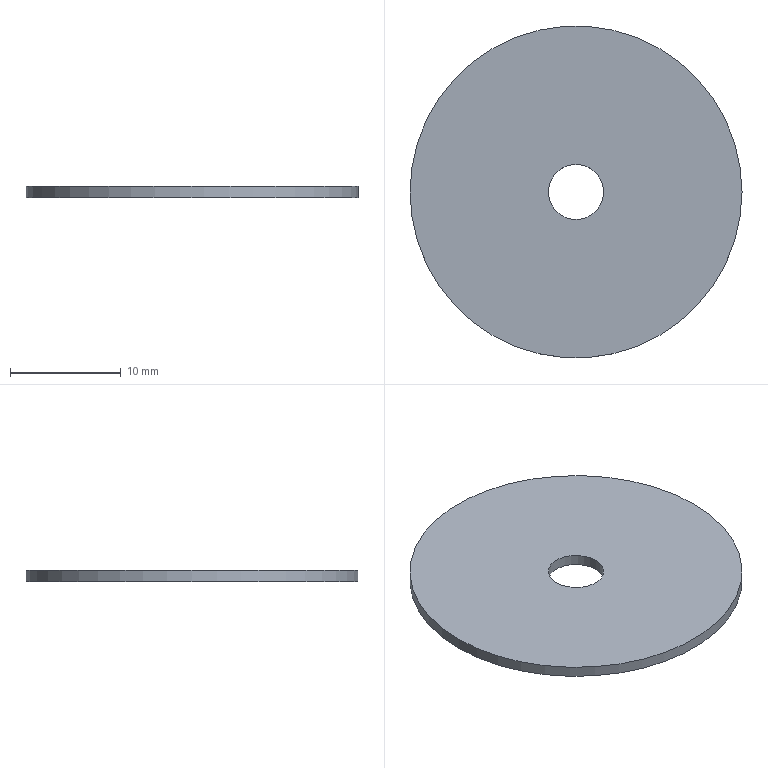Part | NX | features DATUM_CSYS 2, EXTRUDE 1, SKETCH 1 | 1 solid | 4 faces | box 30 x 30 x 1 mm | volume 687.223 mm3 | cylinder 2 | plane 2 | commonest cylinder face diameters 5 x1 30 x1
STEP:
#1=CARTESIAN_POINT('',(15.,0.,1.));
#2=VERTEX_POINT('',#1);
#3=CARTESIAN_POINT('',(0.,0.,1.));
#4=DIRECTION('',(0.,0.,1.));
#5=DIRECTION('',(1.,0.,0.));
#6=AXIS2_PLACEMENT_3D('',#3,#4,#5);
#7=CIRCLE('',#6,15.);
#8=EDGE_CURVE('',#2,#2,#7,.T.);
#9=ORIENTED_EDGE('',*,*,#8,.F.);
#10=EDGE_LOOP('',(#9));
#11=FACE_BOUND('',#10,.T.);
#12=CARTESIAN_POINT('',(15.,0.,0.));
#13=VERTEX_POINT('',#12);
#14=CARTESIAN_POINT('',(0.,0.,0.));
#15=DIRECTION('',(0.,0.,1.));
#16=DIRECTION('',(1.,0.,0.));
#17=AXIS2_PLACEMENT_3D('',#14,#15,#16);
#18=CIRCLE('',#17,15.);
#19=EDGE_CURVE('',#13,#13,#18,.T.);
#20=ORIENTED_EDGE('',*,*,#19,.T.);
#21=EDGE_LOOP('',(#20));
#22=FACE_BOUND('',#21,.T.);
#23=CARTESIAN_POINT('',(0.,0.,1.));
#24=DIRECTION('',(0.,0.,-1.));
#25=DIRECTION('',(-1.,0.,0.));
#26=AXIS2_PLACEMENT_3D('',#23,#24,#25);
#27=CYLINDRICAL_SURFACE('',#26,15.);
#28=ADVANCED_FACE('',(#11,#22),#27,.T.);
#29=CARTESIAN_POINT('',(2.5,0.,1.));
#30=VERTEX_POINT('',#29);
#31=CARTESIAN_POINT('',(0.,0.,1.));
#32=DIRECTION('',(0.,0.,1.));
#33=DIRECTION('',(1.,0.,0.));
#34=AXIS2_PLACEMENT_3D('',#31,#32,#33);
#35=CIRCLE('',#34,2.5);
#36=EDGE_CURVE('',#30,#30,#35,.T.);
#37=ORIENTED_EDGE('',*,*,#36,.T.);
#38=EDGE_LOOP('',(#37));
#39=FACE_BOUND('',#38,.T.);
#40=CARTESIAN_POINT('',(2.5,0.,0.));
#41=VERTEX_POINT('',#40);
#42=CARTESIAN_POINT('',(0.,0.,0.));
#43=DIRECTION('',(0.,0.,1.));
#44=DIRECTION('',(1.,0.,0.));
#45=AXIS2_PLACEMENT_3D('',#42,#43,#44);
#46=CIRCLE('',#45,2.5);
#47=EDGE_CURVE('',#41,#41,#46,.T.);
#48=ORIENTED_EDGE('',*,*,#47,.F.);
#49=EDGE_LOOP('',(#48));
#50=FACE_BOUND('',#49,.T.);
#51=CARTESIAN_POINT('',(0.,0.,1.));
#52=DIRECTION('',(0.,0.,-1.));
#53=DIRECTION('',(-1.,0.,0.));
#54=AXIS2_PLACEMENT_3D('',#51,#52,#53);
#55=CYLINDRICAL_SURFACE('',#54,2.5);
#56=ADVANCED_FACE('',(#39,#50),#55,.F.);
#57=ORIENTED_EDGE('',*,*,#8,.T.);
#58=EDGE_LOOP('',(#57));
#59=FACE_BOUND('',#58,.T.);
#60=ORIENTED_EDGE('',*,*,#36,.F.);
#61=EDGE_LOOP('',(#60));
#62=FACE_BOUND('',#61,.T.);
#63=CARTESIAN_POINT('',(0.,0.,1.));
#64=DIRECTION('',(0.,0.,1.));
#65=DIRECTION('',(1.,0.,0.));
#66=AXIS2_PLACEMENT_3D('',#63,#64,#65);
#67=PLANE('',#66);
#68=ADVANCED_FACE('',(#59,#62),#67,.T.);
#69=ORIENTED_EDGE('',*,*,#19,.F.);
#70=EDGE_LOOP('',(#69));
#71=FACE_BOUND('',#70,.T.);
#72=ORIENTED_EDGE('',*,*,#47,.T.);
#73=EDGE_LOOP('',(#72));
#74=FACE_BOUND('',#73,.T.);
#75=CARTESIAN_POINT('',(0.,0.,0.));
#76=DIRECTION('',(0.,0.,1.));
#77=DIRECTION('',(1.,0.,0.));
#78=AXIS2_PLACEMENT_3D('',#75,#76,#77);
#79=PLANE('',#78);
#80=ADVANCED_FACE('',(#71,#74),#79,.F.);
#81=CLOSED_SHELL('',(#28,#56,#68,#80));
#82=MANIFOLD_SOLID_BREP('',#81);
#83=(LENGTH_UNIT()NAMED_UNIT(*)SI_UNIT(.MILLI.,.METRE.));
#84=UNCERTAINTY_MEASURE_WITH_UNIT(LENGTH_MEASURE(0.00001),#83,'','');
#85=(NAMED_UNIT(*)PLANE_ANGLE_UNIT()SI_UNIT($,.RADIAN.));
#86=(NAMED_UNIT(*)SI_UNIT($,.STERADIAN.)SOLID_ANGLE_UNIT());
#87=(GEOMETRIC_REPRESENTATION_CONTEXT(3)GLOBAL_UNCERTAINTY_ASSIGNED_CONTEXT((#84))GLOBAL_UNIT_ASSIGNED_CONTEXT((#83,#85,#86))REPRESENTATION_CONTEXT('',''));
#88=ADVANCED_BREP_SHAPE_REPRESENTATION('',(#82),#87);